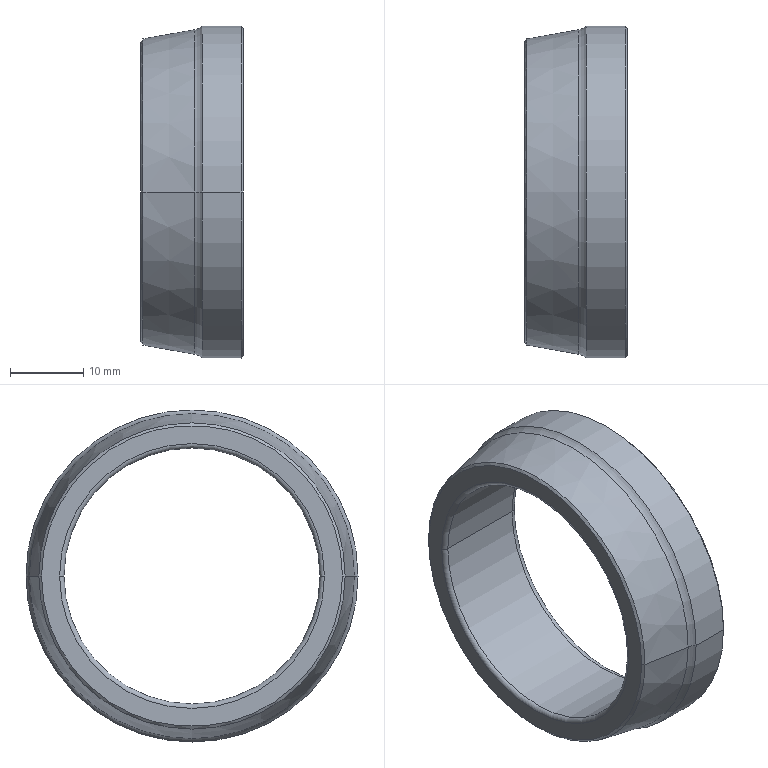Part | SolidWorks | 1 solid | 18 faces | box 14 x 45.385 x 45.385 mm | volume 7900 mm3 | torus 6 | cone 6 | cylinder 4 | plane 2 | commonest cylinder face diameters 35 x2 45.385 x2
STEP:
#1=CARTESIAN_POINT('',(14.,-18.5,0.));
#2=VERTEX_POINT('',#1);
#3=CARTESIAN_POINT('',(13.,-17.5,0.));
#4=VERTEX_POINT('',#3);
#5=CARTESIAN_POINT('',(13.,-18.5,0.));
#6=DIRECTION('',(0.,0.,1.));
#7=DIRECTION('',(1.,0.,0.));
#8=AXIS2_PLACEMENT_3D('',#5,#6,#7);
#9=CIRCLE('',#8,1.);
#10=EDGE_CURVE('',#2,#4,#9,.T.);
#11=ORIENTED_EDGE('',*,*,#10,.F.);
#12=CARTESIAN_POINT('',(14.,18.5,0.));
#13=VERTEX_POINT('',#12);
#14=CARTESIAN_POINT('',(14.,0.,0.));
#15=DIRECTION('',(1.,0.,0.));
#16=DIRECTION('',(0.,-1.,0.));
#17=AXIS2_PLACEMENT_3D('',#14,#15,#16);
#18=CIRCLE('',#17,18.5);
#19=EDGE_CURVE('',#2,#13,#18,.T.);
#20=ORIENTED_EDGE('',*,*,#19,.T.);
#21=CARTESIAN_POINT('',(13.,17.5,0.));
#22=VERTEX_POINT('',#21);
#23=CARTESIAN_POINT('',(13.,18.5,0.));
#24=DIRECTION('',(0.,0.,-1.));
#25=DIRECTION('',(1.,0.,0.));
#26=AXIS2_PLACEMENT_3D('',#23,#24,#25);
#27=CIRCLE('',#26,1.);
#28=EDGE_CURVE('',#13,#22,#27,.T.);
#29=ORIENTED_EDGE('',*,*,#28,.T.);
#30=CARTESIAN_POINT('',(13.,0.,0.));
#31=DIRECTION('',(1.,0.,0.));
#32=DIRECTION('',(0.,-1.,0.));
#33=AXIS2_PLACEMENT_3D('',#30,#31,#32);
#34=CIRCLE('',#33,17.5);
#35=EDGE_CURVE('',#4,#22,#34,.T.);
#36=ORIENTED_EDGE('',*,*,#35,.F.);
#37=EDGE_LOOP('',(#11,#20,#29,#36));
#38=FACE_OUTER_BOUND('',#37,.T.);
#39=CARTESIAN_POINT('',(13.,0.,0.));
#40=DIRECTION('',(1.,0.,0.));
#41=DIRECTION('',(0.,-1.,0.));
#42=AXIS2_PLACEMENT_3D('',#39,#40,#41);
#43=TOROIDAL_SURFACE('',#42,18.5,1.);
#44=ADVANCED_FACE('',(#38),#43,.T.);
#45=CARTESIAN_POINT('',(0.6,-17.5,0.));
#46=VERTEX_POINT('',#45);
#47=CARTESIAN_POINT('',(13.,-17.5,0.));
#48=DIRECTION('',(-1.,0.,0.));
#49=VECTOR('',#48,1000.);
#50=LINE('',#47,#49);
#51=EDGE_CURVE('',#4,#46,#50,.T.);
#52=ORIENTED_EDGE('',*,*,#51,.F.);
#53=ORIENTED_EDGE('',*,*,#35,.T.);
#54=CARTESIAN_POINT('',(0.6,17.5,0.));
#55=VERTEX_POINT('',#54);
#56=CARTESIAN_POINT('',(13.,17.5,0.));
#57=DIRECTION('',(-1.,0.,0.));
#58=VECTOR('',#57,1000.);
#59=LINE('',#56,#58);
#60=EDGE_CURVE('',#22,#55,#59,.T.);
#61=ORIENTED_EDGE('',*,*,#60,.T.);
#62=CARTESIAN_POINT('',(0.6,0.,0.));
#63=DIRECTION('',(-1.,0.,0.));
#64=DIRECTION('',(0.,1.,0.));
#65=AXIS2_PLACEMENT_3D('',#62,#63,#64);
#66=CIRCLE('',#65,17.5);
#67=EDGE_CURVE('',#55,#46,#66,.T.);
#68=ORIENTED_EDGE('',*,*,#67,.T.);
#69=EDGE_LOOP('',(#52,#53,#61,#68));
#70=FACE_OUTER_BOUND('',#69,.T.);
#71=CARTESIAN_POINT('',(0.,0.,0.));
#72=DIRECTION('',(1.,0.,0.));
#73=DIRECTION('',(0.,-1.,0.));
#74=AXIS2_PLACEMENT_3D('',#71,#72,#73);
#75=CYLINDRICAL_SURFACE('',#74,17.5);
#76=ADVANCED_FACE('',(#70),#75,.F.);
#77=CARTESIAN_POINT('',(0.,-18.1,0.));
#78=VERTEX_POINT('',#77);
#79=CARTESIAN_POINT('',(0.6,-18.1,0.));
#80=DIRECTION('',(0.,0.,1.));
#81=DIRECTION('',(0.,1.,0.));
#82=AXIS2_PLACEMENT_3D('',#79,#80,#81);
#83=CIRCLE('',#82,0.6);
#84=EDGE_CURVE('',#46,#78,#83,.T.);
#85=ORIENTED_EDGE('',*,*,#84,.T.);
#86=CARTESIAN_POINT('',(0.,18.1,0.));
#87=VERTEX_POINT('',#86);
#88=CARTESIAN_POINT('',(0.,0.,0.));
#89=DIRECTION('',(-1.,0.,0.));
#90=DIRECTION('',(0.,-1.,0.));
#91=AXIS2_PLACEMENT_3D('',#88,#89,#90);
#92=CIRCLE('',#91,18.1);
#93=EDGE_CURVE('',#78,#87,#92,.T.);
#94=ORIENTED_EDGE('',*,*,#93,.T.);
#95=CARTESIAN_POINT('',(0.6,18.1,0.));
#96=DIRECTION('',(0.,0.,-1.));
#97=DIRECTION('',(0.,-1.,0.));
#98=AXIS2_PLACEMENT_3D('',#95,#96,#97);
#99=CIRCLE('',#98,0.6);
#100=EDGE_CURVE('',#55,#87,#99,.T.);
#101=ORIENTED_EDGE('',*,*,#100,.F.);
#102=CARTESIAN_POINT('',(0.6,0.,0.));
#103=DIRECTION('',(-1.,0.,0.));
#104=DIRECTION('',(0.,-1.,0.));
#105=AXIS2_PLACEMENT_3D('',#102,#103,#104);
#106=CIRCLE('',#105,17.5);
#107=EDGE_CURVE('',#46,#55,#106,.T.);
#108=ORIENTED_EDGE('',*,*,#107,.F.);
#109=EDGE_LOOP('',(#85,#94,#101,#108));
#110=FACE_OUTER_BOUND('',#109,.T.);
#111=CARTESIAN_POINT('',(0.6,0.,0.));
#112=DIRECTION('',(1.,0.,0.));
#113=DIRECTION('',(0.,-1.,0.));
#114=AXIS2_PLACEMENT_3D('',#111,#112,#113);
#115=TOROIDAL_SURFACE('',#114,18.1,0.6);
#116=ADVANCED_FACE('',(#110),#115,.T.);
#117=ORIENTED_EDGE('',*,*,#84,.F.);
#118=ORIENTED_EDGE('',*,*,#67,.F.);
#119=ORIENTED_EDGE('',*,*,#100,.T.);
#120=CARTESIAN_POINT('',(0.,0.,0.));
#121=DIRECTION('',(-1.,0.,0.));
#122=DIRECTION('',(0.,1.,0.));
#123=AXIS2_PLACEMENT_3D('',#120,#121,#122);
#124=CIRCLE('',#123,18.1);
#125=EDGE_CURVE('',#87,#78,#124,.T.);
#126=ORIENTED_EDGE('',*,*,#125,.T.);
#127=EDGE_LOOP('',(#117,#118,#119,#126));
#128=FACE_OUTER_BOUND('',#127,.T.);
#129=CARTESIAN_POINT('',(0.6,0.,0.));
#130=DIRECTION('',(1.,0.,0.));
#131=DIRECTION('',(0.,-1.,0.));
#132=AXIS2_PLACEMENT_3D('',#129,#130,#131);
#133=TOROIDAL_SURFACE('',#132,18.1,0.6);
#134=ADVANCED_FACE('',(#128),#133,.T.);
#135=CARTESIAN_POINT('',(8.408,-22.692,0.));
#136=VERTEX_POINT('',#135);
#137=CARTESIAN_POINT('',(13.7,-22.692,0.));
#138=VERTEX_POINT('',#137);
#139=CARTESIAN_POINT('',(8.408,-22.692,0.));
#140=DIRECTION('',(1.,0.,0.));
#141=VECTOR('',#140,1000.);
#142=LINE('',#139,#141);
#143=EDGE_CURVE('',#136,#138,#142,.T.);
#144=ORIENTED_EDGE('',*,*,#143,.F.);
#145=CARTESIAN_POINT('',(8.408,22.692,0.));
#146=VERTEX_POINT('',#145);
#147=CARTESIAN_POINT('',(8.408,0.,0.));
#148=DIRECTION('',(1.,0.,0.));
#149=DIRECTION('',(0.,-1.,0.));
#150=AXIS2_PLACEMENT_3D('',#147,#148,#149);
#151=CIRCLE('',#150,22.692);
#152=EDGE_CURVE('',#136,#146,#151,.T.);
#153=ORIENTED_EDGE('',*,*,#152,.T.);
#154=CARTESIAN_POINT('',(13.7,22.692,0.));
#155=VERTEX_POINT('',#154);
#156=CARTESIAN_POINT('',(8.408,22.692,0.));
#157=DIRECTION('',(1.,0.,0.));
#158=VECTOR('',#157,1000.);
#159=LINE('',#156,#158);
#160=EDGE_CURVE('',#146,#155,#159,.T.);
#161=ORIENTED_EDGE('',*,*,#160,.T.);
#162=CARTESIAN_POINT('',(13.7,0.,0.));
#163=DIRECTION('',(-1.,0.,0.));
#164=DIRECTION('',(0.,1.,0.));
#165=AXIS2_PLACEMENT_3D('',#162,#163,#164);
#166=CIRCLE('',#165,22.692);
#167=EDGE_CURVE('',#155,#138,#166,.T.);
#168=ORIENTED_EDGE('',*,*,#167,.T.);
#169=EDGE_LOOP('',(#144,#153,#161,#168));
#170=FACE_OUTER_BOUND('',#169,.T.);
#171=CARTESIAN_POINT('',(0.,0.,0.));
#172=DIRECTION('',(1.,0.,0.));
#173=DIRECTION('',(0.,-1.,0.));
#174=AXIS2_PLACEMENT_3D('',#171,#172,#173);
#175=CYLINDRICAL_SURFACE('',#174,22.692);
#176=ADVANCED_FACE('',(#170),#175,.T.);
#177=CARTESIAN_POINT('',(7.367,-22.182,0.));
#178=VERTEX_POINT('',#177);
#179=CARTESIAN_POINT('',(7.,-24.25,0.));
#180=DIRECTION('',(0.,0.,-1.));
#181=DIRECTION('',(0.1747,0.9846,0.));
#182=AXIS2_PLACEMENT_3D('',#179,#180,#181);
#183=CIRCLE('',#182,2.1);
#184=EDGE_CURVE('',#178,#136,#183,.T.);
#185=ORIENTED_EDGE('',*,*,#184,.F.);
#186=CARTESIAN_POINT('',(7.367,22.182,0.));
#187=VERTEX_POINT('',#186);
#188=CARTESIAN_POINT('',(7.367,0.,0.));
#189=DIRECTION('',(-1.,0.,0.));
#190=DIRECTION('',(0.,1.,0.));
#191=AXIS2_PLACEMENT_3D('',#188,#189,#190);
#192=CIRCLE('',#191,22.182);
#193=EDGE_CURVE('',#187,#178,#192,.T.);
#194=ORIENTED_EDGE('',*,*,#193,.F.);
#195=CARTESIAN_POINT('',(7.,24.25,0.));
#196=DIRECTION('',(0.,0.,1.));
#197=DIRECTION('',(0.1747,-0.9846,0.));
#198=AXIS2_PLACEMENT_3D('',#195,#196,#197);
#199=CIRCLE('',#198,2.1);
#200=EDGE_CURVE('',#187,#146,#199,.T.);
#201=ORIENTED_EDGE('',*,*,#200,.T.);
#202=ORIENTED_EDGE('',*,*,#152,.F.);
#203=EDGE_LOOP('',(#185,#194,#201,#202));
#204=FACE_OUTER_BOUND('',#203,.T.);
#205=CARTESIAN_POINT('',(7.,0.,0.));
#206=DIRECTION('',(1.,0.,0.));
#207=DIRECTION('',(0.,-1.,0.));
#208=AXIS2_PLACEMENT_3D('',#205,#206,#207);
#209=TOROIDAL_SURFACE('',#208,24.25,2.1);
#210=ADVANCED_FACE('',(#204),#209,.F.);
#211=CARTESIAN_POINT('',(0.2954,-20.927,0.));
#212=VERTEX_POINT('',#211);
#213=CARTESIAN_POINT('',(0.2954,-20.927,0.));
#214=DIRECTION('',(0.9846,-0.1747,0.));
#215=VECTOR('',#214,1000.);
#216=LINE('',#213,#215);
#217=EDGE_CURVE('',#212,#178,#216,.T.);
#218=ORIENTED_EDGE('',*,*,#217,.F.);
#219=CARTESIAN_POINT('',(0.2954,20.927,0.));
#220=VERTEX_POINT('',#219);
#221=CARTESIAN_POINT('',(0.2954,0.,0.));
#222=DIRECTION('',(1.,0.,0.));
#223=DIRECTION('',(0.,-1.,0.));
#224=AXIS2_PLACEMENT_3D('',#221,#222,#223);
#225=CIRCLE('',#224,20.927);
#226=EDGE_CURVE('',#212,#220,#225,.T.);
#227=ORIENTED_EDGE('',*,*,#226,.T.);
#228=CARTESIAN_POINT('',(0.2954,20.927,0.));
#229=DIRECTION('',(0.9846,0.1747,0.));
#230=VECTOR('',#229,1000.);
#231=LINE('',#228,#230);
#232=EDGE_CURVE('',#220,#187,#231,.T.);
#233=ORIENTED_EDGE('',*,*,#232,.T.);
#234=ORIENTED_EDGE('',*,*,#193,.T.);
#235=EDGE_LOOP('',(#218,#227,#233,#234));
#236=FACE_OUTER_BOUND('',#235,.T.);
#237=CARTESIAN_POINT('',(0.154,0.,0.));
#238=DIRECTION('',(1.,0.,0.));
#239=DIRECTION('',(0.,-1.,0.));
#240=AXIS2_PLACEMENT_3D('',#237,#238,#239);
#241=CONICAL_SURFACE('',#240,20.902,0.1756);
#242=ADVANCED_FACE('',(#236),#241,.T.);
#243=CARTESIAN_POINT('',(0.,-20.575,0.));
#244=VERTEX_POINT('',#243);
#245=CARTESIAN_POINT('',(0.,-20.575,0.));
#246=DIRECTION('',(0.6424,-0.7664,0.));
#247=VECTOR('',#246,1000.);
#248=LINE('',#245,#247);
#249=EDGE_CURVE('',#244,#212,#248,.T.);
#250=ORIENTED_EDGE('',*,*,#249,.F.);
#251=CARTESIAN_POINT('',(0.,20.575,0.));
#252=VERTEX_POINT('',#251);
#253=CARTESIAN_POINT('',(0.,0.,0.));
#254=DIRECTION('',(1.,0.,0.));
#255=DIRECTION('',(0.,-1.,0.));
#256=AXIS2_PLACEMENT_3D('',#253,#254,#255);
#257=CIRCLE('',#256,20.575);
#258=EDGE_CURVE('',#244,#252,#257,.T.);
#259=ORIENTED_EDGE('',*,*,#258,.T.);
#260=CARTESIAN_POINT('',(0.,20.575,0.));
#261=DIRECTION('',(0.6424,0.7664,0.));
#262=VECTOR('',#261,1000.);
#263=LINE('',#260,#262);
#264=EDGE_CURVE('',#252,#220,#263,.T.);
#265=ORIENTED_EDGE('',*,*,#264,.T.);
#266=ORIENTED_EDGE('',*,*,#226,.F.);
#267=EDGE_LOOP('',(#250,#259,#265,#266));
#268=FACE_OUTER_BOUND('',#267,.T.);
#269=CARTESIAN_POINT('',(-0.05064,0.,0.));
#270=DIRECTION('',(1.,0.,0.));
#271=DIRECTION('',(0.,-1.,0.));
#272=AXIS2_PLACEMENT_3D('',#269,#270,#271);
#273=CONICAL_SURFACE('',#272,20.515,0.8732);
#274=ADVANCED_FACE('',(#268),#273,.T.);
#275=ORIENTED_EDGE('',*,*,#93,.F.);
#276=ORIENTED_EDGE('',*,*,#125,.F.);
#277=EDGE_LOOP('',(#275,#276));
#278=FACE_BOUND('',#277,.T.);
#279=ORIENTED_EDGE('',*,*,#258,.F.);
#280=CARTESIAN_POINT('',(0.,0.,0.));
#281=DIRECTION('',(1.,0.,0.));
#282=DIRECTION('',(0.,1.,0.));
#283=AXIS2_PLACEMENT_3D('',#280,#281,#282);
#284=CIRCLE('',#283,20.575);
#285=EDGE_CURVE('',#252,#244,#284,.T.);
#286=ORIENTED_EDGE('',*,*,#285,.F.);
#287=EDGE_LOOP('',(#279,#286));
#288=FACE_OUTER_BOUND('',#287,.T.);
#289=CARTESIAN_POINT('',(0.,0.,0.));
#290=DIRECTION('',(1.,0.,0.));
#291=DIRECTION('',(0.,1.,0.));
#292=AXIS2_PLACEMENT_3D('',#289,#290,#291);
#293=PLANE('',#292);
#294=ADVANCED_FACE('',(#278,#288),#293,.F.);
#295=ORIENTED_EDGE('',*,*,#249,.T.);
#296=CARTESIAN_POINT('',(0.2954,0.,0.));
#297=DIRECTION('',(-1.,0.,0.));
#298=DIRECTION('',(0.,-1.,0.));
#299=AXIS2_PLACEMENT_3D('',#296,#297,#298);
#300=CIRCLE('',#299,20.927);
#301=EDGE_CURVE('',#212,#220,#300,.T.);
#302=ORIENTED_EDGE('',*,*,#301,.T.);
#303=ORIENTED_EDGE('',*,*,#264,.F.);
#304=ORIENTED_EDGE('',*,*,#285,.T.);
#305=EDGE_LOOP('',(#295,#302,#303,#304));
#306=FACE_OUTER_BOUND('',#305,.T.);
#307=CARTESIAN_POINT('',(-0.05064,0.,0.));
#308=DIRECTION('',(1.,0.,0.));
#309=DIRECTION('',(0.,-1.,0.));
#310=AXIS2_PLACEMENT_3D('',#307,#308,#309);
#311=CONICAL_SURFACE('',#310,20.515,0.8732);
#312=ADVANCED_FACE('',(#306),#311,.T.);
#313=ORIENTED_EDGE('',*,*,#217,.T.);
#314=CARTESIAN_POINT('',(7.367,0.,0.));
#315=DIRECTION('',(-1.,0.,0.));
#316=DIRECTION('',(0.,-1.,0.));
#317=AXIS2_PLACEMENT_3D('',#314,#315,#316);
#318=CIRCLE('',#317,22.182);
#319=EDGE_CURVE('',#178,#187,#318,.T.);
#320=ORIENTED_EDGE('',*,*,#319,.T.);
#321=ORIENTED_EDGE('',*,*,#232,.F.);
#322=ORIENTED_EDGE('',*,*,#301,.F.);
#323=EDGE_LOOP('',(#313,#320,#321,#322));
#324=FACE_OUTER_BOUND('',#323,.T.);
#325=CARTESIAN_POINT('',(0.154,0.,0.));
#326=DIRECTION('',(1.,0.,0.));
#327=DIRECTION('',(0.,-1.,0.));
#328=AXIS2_PLACEMENT_3D('',#325,#326,#327);
#329=CONICAL_SURFACE('',#328,20.902,0.1756);
#330=ADVANCED_FACE('',(#324),#329,.T.);
#331=ORIENTED_EDGE('',*,*,#184,.T.);
#332=CARTESIAN_POINT('',(8.408,0.,0.));
#333=DIRECTION('',(1.,0.,0.));
#334=DIRECTION('',(0.,1.,0.));
#335=AXIS2_PLACEMENT_3D('',#332,#333,#334);
#336=CIRCLE('',#335,22.692);
#337=EDGE_CURVE('',#146,#136,#336,.T.);
#338=ORIENTED_EDGE('',*,*,#337,.F.);
#339=ORIENTED_EDGE('',*,*,#200,.F.);
#340=ORIENTED_EDGE('',*,*,#319,.F.);
#341=EDGE_LOOP('',(#331,#338,#339,#340));
#342=FACE_OUTER_BOUND('',#341,.T.);
#343=CARTESIAN_POINT('',(7.,0.,0.));
#344=DIRECTION('',(1.,0.,0.));
#345=DIRECTION('',(0.,-1.,0.));
#346=AXIS2_PLACEMENT_3D('',#343,#344,#345);
#347=TOROIDAL_SURFACE('',#346,24.25,2.1);
#348=ADVANCED_FACE('',(#342),#347,.F.);
#349=ORIENTED_EDGE('',*,*,#143,.T.);
#350=CARTESIAN_POINT('',(13.7,0.,0.));
#351=DIRECTION('',(-1.,0.,0.));
#352=DIRECTION('',(0.,-1.,0.));
#353=AXIS2_PLACEMENT_3D('',#350,#351,#352);
#354=CIRCLE('',#353,22.692);
#355=EDGE_CURVE('',#138,#155,#354,.T.);
#356=ORIENTED_EDGE('',*,*,#355,.T.);
#357=ORIENTED_EDGE('',*,*,#160,.F.);
#358=ORIENTED_EDGE('',*,*,#337,.T.);
#359=EDGE_LOOP('',(#349,#356,#357,#358));
#360=FACE_OUTER_BOUND('',#359,.T.);
#361=CARTESIAN_POINT('',(0.,0.,0.));
#362=DIRECTION('',(1.,0.,0.));
#363=DIRECTION('',(0.,-1.,0.));
#364=AXIS2_PLACEMENT_3D('',#361,#362,#363);
#365=CYLINDRICAL_SURFACE('',#364,22.692);
#366=ADVANCED_FACE('',(#360),#365,.T.);
#367=CARTESIAN_POINT('',(14.,-22.392,0.));
#368=VERTEX_POINT('',#367);
#369=CARTESIAN_POINT('',(13.7,-22.692,0.));
#370=DIRECTION('',(0.7071,0.7071,0.));
#371=VECTOR('',#370,1000.);
#372=LINE('',#369,#371);
#373=EDGE_CURVE('',#138,#368,#372,.T.);
#374=ORIENTED_EDGE('',*,*,#373,.T.);
#375=CARTESIAN_POINT('',(14.,22.392,0.));
#376=VERTEX_POINT('',#375);
#377=CARTESIAN_POINT('',(14.,0.,0.));
#378=DIRECTION('',(-1.,0.,0.));
#379=DIRECTION('',(0.,-1.,0.));
#380=AXIS2_PLACEMENT_3D('',#377,#378,#379);
#381=CIRCLE('',#380,22.392);
#382=EDGE_CURVE('',#368,#376,#381,.T.);
#383=ORIENTED_EDGE('',*,*,#382,.T.);
#384=CARTESIAN_POINT('',(13.7,22.692,0.));
#385=DIRECTION('',(0.7071,-0.7071,0.));
#386=VECTOR('',#385,1000.);
#387=LINE('',#384,#386);
#388=EDGE_CURVE('',#155,#376,#387,.T.);
#389=ORIENTED_EDGE('',*,*,#388,.F.);
#390=ORIENTED_EDGE('',*,*,#355,.F.);
#391=EDGE_LOOP('',(#374,#383,#389,#390));
#392=FACE_OUTER_BOUND('',#391,.T.);
#393=CARTESIAN_POINT('',(14.056,0.,0.));
#394=DIRECTION('',(-1.,0.,0.));
#395=DIRECTION('',(0.,1.,0.));
#396=AXIS2_PLACEMENT_3D('',#393,#394,#395);
#397=CONICAL_SURFACE('',#396,22.337,0.7854);
#398=ADVANCED_FACE('',(#392),#397,.T.);
#399=ORIENTED_EDGE('',*,*,#373,.F.);
#400=ORIENTED_EDGE('',*,*,#167,.F.);
#401=ORIENTED_EDGE('',*,*,#388,.T.);
#402=CARTESIAN_POINT('',(14.,0.,0.));
#403=DIRECTION('',(-1.,0.,0.));
#404=DIRECTION('',(0.,1.,0.));
#405=AXIS2_PLACEMENT_3D('',#402,#403,#404);
#406=CIRCLE('',#405,22.392);
#407=EDGE_CURVE('',#376,#368,#406,.T.);
#408=ORIENTED_EDGE('',*,*,#407,.T.);
#409=EDGE_LOOP('',(#399,#400,#401,#408));
#410=FACE_OUTER_BOUND('',#409,.T.);
#411=CARTESIAN_POINT('',(14.056,0.,0.));
#412=DIRECTION('',(-1.,0.,0.));
#413=DIRECTION('',(0.,1.,0.));
#414=AXIS2_PLACEMENT_3D('',#411,#412,#413);
#415=CONICAL_SURFACE('',#414,22.337,0.7854);
#416=ADVANCED_FACE('',(#410),#415,.T.);
#417=ORIENTED_EDGE('',*,*,#19,.F.);
#418=CARTESIAN_POINT('',(14.,0.,0.));
#419=DIRECTION('',(1.,0.,0.));
#420=DIRECTION('',(0.,1.,0.));
#421=AXIS2_PLACEMENT_3D('',#418,#419,#420);
#422=CIRCLE('',#421,18.5);
#423=EDGE_CURVE('',#13,#2,#422,.T.);
#424=ORIENTED_EDGE('',*,*,#423,.F.);
#425=EDGE_LOOP('',(#417,#424));
#426=FACE_BOUND('',#425,.T.);
#427=ORIENTED_EDGE('',*,*,#382,.F.);
#428=ORIENTED_EDGE('',*,*,#407,.F.);
#429=EDGE_LOOP('',(#427,#428));
#430=FACE_OUTER_BOUND('',#429,.T.);
#431=CARTESIAN_POINT('',(14.,0.,0.));
#432=DIRECTION('',(1.,0.,0.));
#433=DIRECTION('',(0.,1.,0.));
#434=AXIS2_PLACEMENT_3D('',#431,#432,#433);
#435=PLANE('',#434);
#436=ADVANCED_FACE('',(#426,#430),#435,.T.);
#437=ORIENTED_EDGE('',*,*,#10,.T.);
#438=CARTESIAN_POINT('',(13.,0.,0.));
#439=DIRECTION('',(1.,0.,0.));
#440=DIRECTION('',(0.,1.,0.));
#441=AXIS2_PLACEMENT_3D('',#438,#439,#440);
#442=CIRCLE('',#441,17.5);
#443=EDGE_CURVE('',#22,#4,#442,.T.);
#444=ORIENTED_EDGE('',*,*,#443,.F.);
#445=ORIENTED_EDGE('',*,*,#28,.F.);
#446=ORIENTED_EDGE('',*,*,#423,.T.);
#447=EDGE_LOOP('',(#437,#444,#445,#446));
#448=FACE_OUTER_BOUND('',#447,.T.);
#449=CARTESIAN_POINT('',(13.,0.,0.));
#450=DIRECTION('',(1.,0.,0.));
#451=DIRECTION('',(0.,-1.,0.));
#452=AXIS2_PLACEMENT_3D('',#449,#450,#451);
#453=TOROIDAL_SURFACE('',#452,18.5,1.);
#454=ADVANCED_FACE('',(#448),#453,.T.);
#455=ORIENTED_EDGE('',*,*,#51,.T.);
#456=ORIENTED_EDGE('',*,*,#107,.T.);
#457=ORIENTED_EDGE('',*,*,#60,.F.);
#458=ORIENTED_EDGE('',*,*,#443,.T.);
#459=EDGE_LOOP('',(#455,#456,#457,#458));
#460=FACE_OUTER_BOUND('',#459,.T.);
#461=CARTESIAN_POINT('',(0.,0.,0.));
#462=DIRECTION('',(1.,0.,0.));
#463=DIRECTION('',(0.,-1.,0.));
#464=AXIS2_PLACEMENT_3D('',#461,#462,#463);
#465=CYLINDRICAL_SURFACE('',#464,17.5);
#466=ADVANCED_FACE('',(#460),#465,.F.);
#467=CLOSED_SHELL('',(#44,#76,#116,#134,#176,#210,#242,#274,#294,#312,#330,#348,#366,#398,#416,#436,#454,#466));
#468=MANIFOLD_SOLID_BREP('',#467);
#469=CARTESIAN_POINT('',(0.,0.,0.));
#470=DIRECTION('',(0.,0.,1.));
#471=DIRECTION('',(1.,0.,0.));
#472=AXIS2_PLACEMENT_3D('',#469,#470,#471);
#473=(LENGTH_UNIT()NAMED_UNIT(*)SI_UNIT(.MILLI.,.METRE.));
#474=UNCERTAINTY_MEASURE_WITH_UNIT(LENGTH_MEASURE(0.00001),#473,'','');
#475=(NAMED_UNIT(*)PLANE_ANGLE_UNIT()SI_UNIT($,.RADIAN.));
#476=(NAMED_UNIT(*)SI_UNIT($,.STERADIAN.)SOLID_ANGLE_UNIT());
#477=(GEOMETRIC_REPRESENTATION_CONTEXT(3)GLOBAL_UNCERTAINTY_ASSIGNED_CONTEXT((#474))GLOBAL_UNIT_ASSIGNED_CONTEXT((#473,#475,#476))REPRESENTATION_CONTEXT('',''));
#478=ADVANCED_BREP_SHAPE_REPRESENTATION('',(#468,#472),#477);